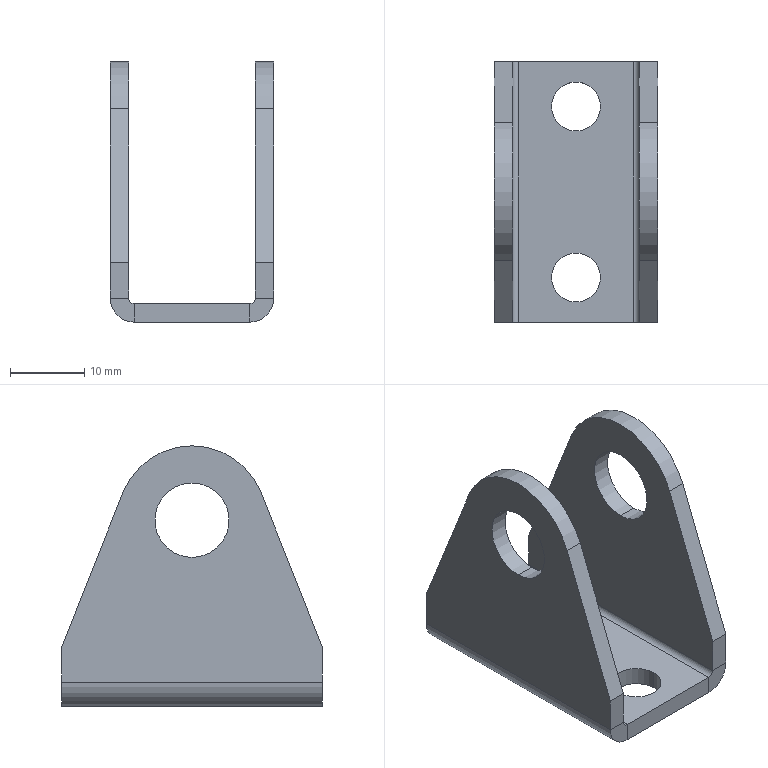Part | NX | features BREP 1 | 1 solid | 34 faces | box 22 x 35 x 35 mm | volume 5371 mm3 | plane 20 | cylinder 14 | commonest cylinder face diameters 6.6 x4 10 x4 1.473 x2 6.473 x2 20 x2
STEP:
#1=CARTESIAN_POINT('',(-3.3,-11.5,-2.5));
#2=VERTEX_POINT('',#1);
#3=CARTESIAN_POINT('',(3.3,-11.5,-2.5));
#4=VERTEX_POINT('',#3);
#5=CARTESIAN_POINT('',(0.,-11.5,-2.5));
#6=DIRECTION('',(0.,0.,1.));
#7=DIRECTION('',(1.,0.,0.));
#8=AXIS2_PLACEMENT_3D('',#5,#6,#7);
#9=CIRCLE('',#8,3.3);
#10=EDGE_CURVE('',#2,#4,#9,.T.);
#11=ORIENTED_EDGE('',*,*,#10,.F.);
#12=CARTESIAN_POINT('',(-3.3,-11.5,0.));
#13=VERTEX_POINT('',#12);
#14=CARTESIAN_POINT('',(-3.3,-11.5,0.));
#15=DIRECTION('',(0.,0.,1.));
#16=VECTOR('',#15,1000.);
#17=LINE('',#14,#16);
#18=EDGE_CURVE('',#13,#2,#17,.F.);
#19=ORIENTED_EDGE('',*,*,#18,.F.);
#20=CARTESIAN_POINT('',(3.3,-11.5,0.));
#21=VERTEX_POINT('',#20);
#22=CARTESIAN_POINT('',(0.,-11.5,0.));
#23=DIRECTION('',(0.,0.,1.));
#24=DIRECTION('',(1.,0.,0.));
#25=AXIS2_PLACEMENT_3D('',#22,#23,#24);
#26=CIRCLE('',#25,3.3);
#27=EDGE_CURVE('',#13,#21,#26,.T.);
#28=ORIENTED_EDGE('',*,*,#27,.T.);
#29=CARTESIAN_POINT('',(3.3,-11.5,0.));
#30=DIRECTION('',(0.,0.,1.));
#31=VECTOR('',#30,1000.);
#32=LINE('',#29,#31);
#33=EDGE_CURVE('',#21,#4,#32,.F.);
#34=ORIENTED_EDGE('',*,*,#33,.T.);
#35=EDGE_LOOP('',(#11,#19,#28,#34));
#36=FACE_BOUND('',#35,.T.);
#37=CARTESIAN_POINT('',(0.,-11.5,0.));
#38=DIRECTION('',(0.,0.,1.));
#39=DIRECTION('',(1.,0.,0.));
#40=AXIS2_PLACEMENT_3D('',#37,#38,#39);
#41=CYLINDRICAL_SURFACE('',#40,3.3);
#42=ADVANCED_FACE('',(#36),#41,.F.);
#43=CARTESIAN_POINT('',(-3.3,11.5,-2.5));
#44=VERTEX_POINT('',#43);
#45=CARTESIAN_POINT('',(3.3,11.5,-2.5));
#46=VERTEX_POINT('',#45);
#47=CARTESIAN_POINT('',(0.,11.5,-2.5));
#48=DIRECTION('',(0.,0.,1.));
#49=DIRECTION('',(1.,0.,0.));
#50=AXIS2_PLACEMENT_3D('',#47,#48,#49);
#51=CIRCLE('',#50,3.3);
#52=EDGE_CURVE('',#44,#46,#51,.T.);
#53=ORIENTED_EDGE('',*,*,#52,.F.);
#54=CARTESIAN_POINT('',(-3.3,11.5,0.));
#55=VERTEX_POINT('',#54);
#56=CARTESIAN_POINT('',(-3.3,11.5,0.));
#57=DIRECTION('',(0.,0.,1.));
#58=VECTOR('',#57,1000.);
#59=LINE('',#56,#58);
#60=EDGE_CURVE('',#55,#44,#59,.F.);
#61=ORIENTED_EDGE('',*,*,#60,.F.);
#62=CARTESIAN_POINT('',(3.3,11.5,0.));
#63=VERTEX_POINT('',#62);
#64=CARTESIAN_POINT('',(0.,11.5,0.));
#65=DIRECTION('',(0.,0.,1.));
#66=DIRECTION('',(1.,0.,0.));
#67=AXIS2_PLACEMENT_3D('',#64,#65,#66);
#68=CIRCLE('',#67,3.3);
#69=EDGE_CURVE('',#55,#63,#68,.T.);
#70=ORIENTED_EDGE('',*,*,#69,.T.);
#71=CARTESIAN_POINT('',(3.3,11.5,0.));
#72=DIRECTION('',(0.,0.,1.));
#73=VECTOR('',#72,1000.);
#74=LINE('',#71,#73);
#75=EDGE_CURVE('',#63,#46,#74,.F.);
#76=ORIENTED_EDGE('',*,*,#75,.T.);
#77=EDGE_LOOP('',(#53,#61,#70,#76));
#78=FACE_BOUND('',#77,.T.);
#79=CARTESIAN_POINT('',(0.,11.5,0.));
#80=DIRECTION('',(0.,0.,1.));
#81=DIRECTION('',(1.,0.,0.));
#82=AXIS2_PLACEMENT_3D('',#79,#80,#81);
#83=CYLINDRICAL_SURFACE('',#82,3.3);
#84=ADVANCED_FACE('',(#78),#83,.F.);
#85=CARTESIAN_POINT('',(-11.,0.,27.5));
#86=VERTEX_POINT('',#85);
#87=CARTESIAN_POINT('',(-11.,0.,17.5));
#88=VERTEX_POINT('',#87);
#89=CARTESIAN_POINT('',(-11.,0.,22.5));
#90=DIRECTION('',(1.,0.,0.));
#91=DIRECTION('',(0.,0.,-1.));
#92=AXIS2_PLACEMENT_3D('',#89,#90,#91);
#93=CIRCLE('',#92,5.);
#94=EDGE_CURVE('',#86,#88,#93,.T.);
#95=ORIENTED_EDGE('',*,*,#94,.F.);
#96=CARTESIAN_POINT('',(-8.5,0.,27.5));
#97=VERTEX_POINT('',#96);
#98=CARTESIAN_POINT('',(-29.,0.,27.5));
#99=DIRECTION('',(1.,0.,0.));
#100=VECTOR('',#99,1000.);
#101=LINE('',#98,#100);
#102=EDGE_CURVE('',#86,#97,#101,.T.);
#103=ORIENTED_EDGE('',*,*,#102,.T.);
#104=CARTESIAN_POINT('',(-8.5,0.,17.5));
#105=VERTEX_POINT('',#104);
#106=CARTESIAN_POINT('',(-8.5,0.,22.5));
#107=DIRECTION('',(1.,0.,0.));
#108=DIRECTION('',(0.,0.,-1.));
#109=AXIS2_PLACEMENT_3D('',#106,#107,#108);
#110=CIRCLE('',#109,5.);
#111=EDGE_CURVE('',#97,#105,#110,.T.);
#112=ORIENTED_EDGE('',*,*,#111,.T.);
#113=CARTESIAN_POINT('',(-29.,0.,17.5));
#114=DIRECTION('',(1.,0.,0.));
#115=VECTOR('',#114,1000.);
#116=LINE('',#113,#115);
#117=EDGE_CURVE('',#88,#105,#116,.T.);
#118=ORIENTED_EDGE('',*,*,#117,.F.);
#119=EDGE_LOOP('',(#95,#103,#112,#118));
#120=FACE_BOUND('',#119,.T.);
#121=CARTESIAN_POINT('',(-29.,0.,22.5));
#122=DIRECTION('',(1.,0.,0.));
#123=DIRECTION('',(0.,0.,-1.));
#124=AXIS2_PLACEMENT_3D('',#121,#122,#123);
#125=CYLINDRICAL_SURFACE('',#124,5.);
#126=ADVANCED_FACE('',(#120),#125,.F.);
#127=CARTESIAN_POINT('',(8.5,0.,17.5));
#128=VERTEX_POINT('',#127);
#129=CARTESIAN_POINT('',(8.5,0.,27.5));
#130=VERTEX_POINT('',#129);
#131=CARTESIAN_POINT('',(8.5,0.,22.5));
#132=DIRECTION('',(-1.,0.,0.));
#133=DIRECTION('',(0.,0.,1.));
#134=AXIS2_PLACEMENT_3D('',#131,#132,#133);
#135=CIRCLE('',#134,5.);
#136=EDGE_CURVE('',#128,#130,#135,.T.);
#137=ORIENTED_EDGE('',*,*,#136,.T.);
#138=CARTESIAN_POINT('',(11.,0.,27.5));
#139=VERTEX_POINT('',#138);
#140=CARTESIAN_POINT('',(-29.,0.,27.5));
#141=DIRECTION('',(1.,0.,0.));
#142=VECTOR('',#141,1000.);
#143=LINE('',#140,#142);
#144=EDGE_CURVE('',#130,#139,#143,.T.);
#145=ORIENTED_EDGE('',*,*,#144,.T.);
#146=CARTESIAN_POINT('',(11.,0.,17.5));
#147=VERTEX_POINT('',#146);
#148=CARTESIAN_POINT('',(11.,0.,22.5));
#149=DIRECTION('',(1.,0.,0.));
#150=DIRECTION('',(0.,0.,-1.));
#151=AXIS2_PLACEMENT_3D('',#148,#149,#150);
#152=CIRCLE('',#151,5.);
#153=EDGE_CURVE('',#139,#147,#152,.T.);
#154=ORIENTED_EDGE('',*,*,#153,.T.);
#155=CARTESIAN_POINT('',(-29.,0.,17.5));
#156=DIRECTION('',(1.,0.,0.));
#157=VECTOR('',#156,1000.);
#158=LINE('',#155,#157);
#159=EDGE_CURVE('',#128,#147,#158,.T.);
#160=ORIENTED_EDGE('',*,*,#159,.F.);
#161=EDGE_LOOP('',(#137,#145,#154,#160));
#162=FACE_BOUND('',#161,.T.);
#163=CARTESIAN_POINT('',(-29.,0.,22.5));
#164=DIRECTION('',(1.,0.,0.));
#165=DIRECTION('',(0.,0.,-1.));
#166=AXIS2_PLACEMENT_3D('',#163,#164,#165);
#167=CYLINDRICAL_SURFACE('',#166,5.);
#168=ADVANCED_FACE('',(#162),#167,.F.);
#169=CARTESIAN_POINT('',(7.763,17.5,-2.5));
#170=VERTEX_POINT('',#169);
#171=CARTESIAN_POINT('',(-7.763,17.5,-2.5));
#172=VERTEX_POINT('',#171);
#173=CARTESIAN_POINT('',(-11.,17.5,-2.5));
#174=DIRECTION('',(-1.,0.,0.));
#175=VECTOR('',#174,1000.);
#176=LINE('',#173,#175);
#177=EDGE_CURVE('',#170,#172,#176,.T.);
#178=ORIENTED_EDGE('',*,*,#177,.F.);
#179=CARTESIAN_POINT('',(7.763,-17.5,-2.5));
#180=VERTEX_POINT('',#179);
#181=CARTESIAN_POINT('',(7.763,17.5,-2.5));
#182=DIRECTION('',(0.,-1.,0.));
#183=VECTOR('',#182,1000.);
#184=LINE('',#181,#183);
#185=EDGE_CURVE('',#170,#180,#184,.T.);
#186=ORIENTED_EDGE('',*,*,#185,.T.);
#187=CARTESIAN_POINT('',(-7.763,-17.5,-2.5));
#188=VERTEX_POINT('',#187);
#189=CARTESIAN_POINT('',(-11.,-17.5,-2.5));
#190=DIRECTION('',(1.,0.,0.));
#191=VECTOR('',#190,1000.);
#192=LINE('',#189,#191);
#193=EDGE_CURVE('',#188,#180,#192,.T.);
#194=ORIENTED_EDGE('',*,*,#193,.F.);
#195=CARTESIAN_POINT('',(-7.763,-17.5,-2.5));
#196=DIRECTION('',(0.,1.,0.));
#197=VECTOR('',#196,1000.);
#198=LINE('',#195,#197);
#199=EDGE_CURVE('',#188,#172,#198,.T.);
#200=ORIENTED_EDGE('',*,*,#199,.T.);
#201=EDGE_LOOP('',(#178,#186,#194,#200));
#202=FACE_BOUND('',#201,.T.);
#203=CARTESIAN_POINT('',(0.,11.5,-2.5));
#204=DIRECTION('',(0.,0.,1.));
#205=DIRECTION('',(1.,0.,0.));
#206=AXIS2_PLACEMENT_3D('',#203,#204,#205);
#207=CIRCLE('',#206,3.3);
#208=EDGE_CURVE('',#46,#44,#207,.T.);
#209=ORIENTED_EDGE('',*,*,#208,.T.);
#210=ORIENTED_EDGE('',*,*,#52,.T.);
#211=EDGE_LOOP('',(#209,#210));
#212=FACE_BOUND('',#211,.T.);
#213=CARTESIAN_POINT('',(0.,-11.5,-2.5));
#214=DIRECTION('',(0.,0.,1.));
#215=DIRECTION('',(1.,0.,0.));
#216=AXIS2_PLACEMENT_3D('',#213,#214,#215);
#217=CIRCLE('',#216,3.3);
#218=EDGE_CURVE('',#4,#2,#217,.T.);
#219=ORIENTED_EDGE('',*,*,#218,.T.);
#220=ORIENTED_EDGE('',*,*,#10,.T.);
#221=EDGE_LOOP('',(#219,#220));
#222=FACE_BOUND('',#221,.T.);
#223=CARTESIAN_POINT('',(0.,0.,-2.5));
#224=DIRECTION('',(0.,0.,-1.));
#225=DIRECTION('',(0.,-1.,0.));
#226=AXIS2_PLACEMENT_3D('',#223,#224,#225);
#227=PLANE('',#226);
#228=ADVANCED_FACE('',(#202,#212,#222),#227,.T.);
#229=CARTESIAN_POINT('',(7.763,17.5,0.));
#230=VERTEX_POINT('',#229);
#231=CARTESIAN_POINT('',(7.763,-17.5,0.));
#232=VERTEX_POINT('',#231);
#233=CARTESIAN_POINT('',(7.763,17.5,0.));
#234=DIRECTION('',(0.,-1.,0.));
#235=VECTOR('',#234,1000.);
#236=LINE('',#233,#235);
#237=EDGE_CURVE('',#230,#232,#236,.T.);
#238=ORIENTED_EDGE('',*,*,#237,.F.);
#239=CARTESIAN_POINT('',(-7.763,17.5,0.));
#240=VERTEX_POINT('',#239);
#241=CARTESIAN_POINT('',(-11.,17.5,0.));
#242=DIRECTION('',(-1.,0.,0.));
#243=VECTOR('',#242,1000.);
#244=LINE('',#241,#243);
#245=EDGE_CURVE('',#230,#240,#244,.T.);
#246=ORIENTED_EDGE('',*,*,#245,.T.);
#247=CARTESIAN_POINT('',(-7.763,-17.5,0.));
#248=VERTEX_POINT('',#247);
#249=CARTESIAN_POINT('',(-7.763,-17.5,0.));
#250=DIRECTION('',(0.,1.,0.));
#251=VECTOR('',#250,1000.);
#252=LINE('',#249,#251);
#253=EDGE_CURVE('',#248,#240,#252,.T.);
#254=ORIENTED_EDGE('',*,*,#253,.F.);
#255=CARTESIAN_POINT('',(-11.,-17.5,0.));
#256=DIRECTION('',(1.,0.,0.));
#257=VECTOR('',#256,1000.);
#258=LINE('',#255,#257);
#259=EDGE_CURVE('',#248,#232,#258,.T.);
#260=ORIENTED_EDGE('',*,*,#259,.T.);
#261=EDGE_LOOP('',(#238,#246,#254,#260));
#262=FACE_BOUND('',#261,.T.);
#263=CARTESIAN_POINT('',(0.,-11.5,0.));
#264=DIRECTION('',(0.,0.,1.));
#265=DIRECTION('',(1.,0.,0.));
#266=AXIS2_PLACEMENT_3D('',#263,#264,#265);
#267=CIRCLE('',#266,3.3);
#268=EDGE_CURVE('',#21,#13,#267,.T.);
#269=ORIENTED_EDGE('',*,*,#268,.F.);
#270=ORIENTED_EDGE('',*,*,#27,.F.);
#271=EDGE_LOOP('',(#269,#270));
#272=FACE_BOUND('',#271,.T.);
#273=CARTESIAN_POINT('',(0.,11.5,0.));
#274=DIRECTION('',(0.,0.,1.));
#275=DIRECTION('',(1.,0.,0.));
#276=AXIS2_PLACEMENT_3D('',#273,#274,#275);
#277=CIRCLE('',#276,3.3);
#278=EDGE_CURVE('',#63,#55,#277,.T.);
#279=ORIENTED_EDGE('',*,*,#278,.F.);
#280=ORIENTED_EDGE('',*,*,#69,.F.);
#281=EDGE_LOOP('',(#279,#280));
#282=FACE_BOUND('',#281,.T.);
#283=CARTESIAN_POINT('',(0.,0.,0.));
#284=DIRECTION('',(0.,0.,-1.));
#285=DIRECTION('',(0.,-1.,0.));
#286=AXIS2_PLACEMENT_3D('',#283,#284,#285);
#287=PLANE('',#286);
#288=ADVANCED_FACE('',(#262,#272,#282),#287,.F.);
#289=ORIENTED_EDGE('',*,*,#245,.F.);
#290=CARTESIAN_POINT('',(7.763,17.5,0.));
#291=DIRECTION('',(0.,0.,-1.));
#292=VECTOR('',#291,1000.);
#293=LINE('',#290,#292);
#294=EDGE_CURVE('',#230,#170,#293,.T.);
#295=ORIENTED_EDGE('',*,*,#294,.T.);
#296=ORIENTED_EDGE('',*,*,#177,.T.);
#297=CARTESIAN_POINT('',(-7.763,17.5,0.));
#298=DIRECTION('',(0.,0.,-1.));
#299=VECTOR('',#298,1000.);
#300=LINE('',#297,#299);
#301=EDGE_CURVE('',#240,#172,#300,.T.);
#302=ORIENTED_EDGE('',*,*,#301,.F.);
#303=EDGE_LOOP('',(#289,#295,#296,#302));
#304=FACE_BOUND('',#303,.T.);
#305=CARTESIAN_POINT('',(-11.,17.5,-2.5));
#306=DIRECTION('',(0.,1.,0.));
#307=DIRECTION('',(1.,0.,0.));
#308=AXIS2_PLACEMENT_3D('',#305,#306,#307);
#309=PLANE('',#308);
#310=ADVANCED_FACE('',(#304),#309,.T.);
#311=CARTESIAN_POINT('',(7.763,-17.5,0.));
#312=DIRECTION('',(0.,0.,-1.));
#313=VECTOR('',#312,1000.);
#314=LINE('',#311,#313);
#315=EDGE_CURVE('',#232,#180,#314,.T.);
#316=ORIENTED_EDGE('',*,*,#315,.F.);
#317=ORIENTED_EDGE('',*,*,#259,.F.);
#318=CARTESIAN_POINT('',(-7.763,-17.5,0.));
#319=DIRECTION('',(0.,0.,-1.));
#320=VECTOR('',#319,1000.);
#321=LINE('',#318,#320);
#322=EDGE_CURVE('',#248,#188,#321,.T.);
#323=ORIENTED_EDGE('',*,*,#322,.T.);
#324=ORIENTED_EDGE('',*,*,#193,.T.);
#325=EDGE_LOOP('',(#316,#317,#323,#324));
#326=FACE_BOUND('',#325,.T.);
#327=CARTESIAN_POINT('',(-11.,-17.5,-2.5));
#328=DIRECTION('',(0.,-1.,0.));
#329=DIRECTION('',(0.,0.,-1.));
#330=AXIS2_PLACEMENT_3D('',#327,#328,#329);
#331=PLANE('',#330);
#332=ADVANCED_FACE('',(#326),#331,.T.);
#333=CARTESIAN_POINT('',(-8.5,17.5,0.7366));
#334=VERTEX_POINT('',#333);
#335=CARTESIAN_POINT('',(-11.,17.5,0.7366));
#336=VERTEX_POINT('',#335);
#337=CARTESIAN_POINT('',(-11.,17.5,0.7366));
#338=DIRECTION('',(-1.,0.,0.));
#339=VECTOR('',#338,1000.);
#340=LINE('',#337,#339);
#341=EDGE_CURVE('',#334,#336,#340,.T.);
#342=ORIENTED_EDGE('',*,*,#341,.F.);
#343=CARTESIAN_POINT('',(-7.763,17.5,0.7366));
#344=DIRECTION('',(0.,1.,0.));
#345=DIRECTION('',(0.,0.,-1.));
#346=AXIS2_PLACEMENT_3D('',#343,#344,#345);
#347=CIRCLE('',#346,0.7366);
#348=EDGE_CURVE('',#240,#334,#347,.T.);
#349=ORIENTED_EDGE('',*,*,#348,.F.);
#350=ORIENTED_EDGE('',*,*,#301,.T.);
#351=CARTESIAN_POINT('',(-7.763,17.5,0.7366));
#352=DIRECTION('',(0.,1.,0.));
#353=DIRECTION('',(0.,0.,-1.));
#354=AXIS2_PLACEMENT_3D('',#351,#352,#353);
#355=CIRCLE('',#354,3.237);
#356=EDGE_CURVE('',#172,#336,#355,.T.);
#357=ORIENTED_EDGE('',*,*,#356,.T.);
#358=EDGE_LOOP('',(#342,#349,#350,#357));
#359=FACE_BOUND('',#358,.T.);
#360=CARTESIAN_POINT('',(-7.763,17.5,0.7366));
#361=DIRECTION('',(0.,1.,0.));
#362=DIRECTION('',(1.,0.,0.));
#363=AXIS2_PLACEMENT_3D('',#360,#361,#362);
#364=PLANE('',#363);
#365=ADVANCED_FACE('',(#359),#364,.T.);
#366=CARTESIAN_POINT('',(-8.5,-17.5,0.7366));
#367=VERTEX_POINT('',#366);
#368=CARTESIAN_POINT('',(-7.763,-17.5,0.7366));
#369=DIRECTION('',(0.,-1.,0.));
#370=DIRECTION('',(0.,0.,-1.));
#371=AXIS2_PLACEMENT_3D('',#368,#369,#370);
#372=CIRCLE('',#371,0.7366);
#373=EDGE_CURVE('',#367,#248,#372,.T.);
#374=ORIENTED_EDGE('',*,*,#373,.F.);
#375=CARTESIAN_POINT('',(-11.,-17.5,0.7366));
#376=VERTEX_POINT('',#375);
#377=CARTESIAN_POINT('',(-8.5,-17.5,0.7366));
#378=DIRECTION('',(-1.,0.,0.));
#379=VECTOR('',#378,1000.);
#380=LINE('',#377,#379);
#381=EDGE_CURVE('',#367,#376,#380,.T.);
#382=ORIENTED_EDGE('',*,*,#381,.T.);
#383=CARTESIAN_POINT('',(-7.763,-17.5,0.7366));
#384=DIRECTION('',(0.,-1.,0.));
#385=DIRECTION('',(0.,0.,-1.));
#386=AXIS2_PLACEMENT_3D('',#383,#384,#385);
#387=CIRCLE('',#386,3.237);
#388=EDGE_CURVE('',#376,#188,#387,.T.);
#389=ORIENTED_EDGE('',*,*,#388,.T.);
#390=ORIENTED_EDGE('',*,*,#322,.F.);
#391=EDGE_LOOP('',(#374,#382,#389,#390));
#392=FACE_BOUND('',#391,.T.);
#393=CARTESIAN_POINT('',(-7.763,-17.5,0.7366));
#394=DIRECTION('',(0.,1.,0.));
#395=DIRECTION('',(1.,0.,0.));
#396=AXIS2_PLACEMENT_3D('',#393,#394,#395);
#397=PLANE('',#396);
#398=ADVANCED_FACE('',(#392),#397,.F.);
#399=ORIENTED_EDGE('',*,*,#199,.F.);
#400=ORIENTED_EDGE('',*,*,#388,.F.);
#401=CARTESIAN_POINT('',(-11.,17.5,0.7366));
#402=DIRECTION('',(0.,1.,0.));
#403=VECTOR('',#402,1000.);
#404=LINE('',#401,#403);
#405=EDGE_CURVE('',#376,#336,#404,.T.);
#406=ORIENTED_EDGE('',*,*,#405,.T.);
#407=ORIENTED_EDGE('',*,*,#356,.F.);
#408=EDGE_LOOP('',(#399,#400,#406,#407));
#409=FACE_BOUND('',#408,.T.);
#410=CARTESIAN_POINT('',(-7.763,-17.5,0.7366));
#411=DIRECTION('',(0.,-1.,0.));
#412=DIRECTION('',(-1.,0.,0.));
#413=AXIS2_PLACEMENT_3D('',#410,#411,#412);
#414=CYLINDRICAL_SURFACE('',#413,3.237);
#415=ADVANCED_FACE('',(#409),#414,.T.);
#416=ORIENTED_EDGE('',*,*,#253,.T.);
#417=ORIENTED_EDGE('',*,*,#348,.T.);
#418=CARTESIAN_POINT('',(-8.5,17.5,0.7366));
#419=DIRECTION('',(0.,-1.,0.));
#420=VECTOR('',#419,1000.);
#421=LINE('',#418,#420);
#422=EDGE_CURVE('',#334,#367,#421,.T.);
#423=ORIENTED_EDGE('',*,*,#422,.T.);
#424=ORIENTED_EDGE('',*,*,#373,.T.);
#425=EDGE_LOOP('',(#416,#417,#423,#424));
#426=FACE_BOUND('',#425,.T.);
#427=CARTESIAN_POINT('',(-7.763,-17.5,0.7366));
#428=DIRECTION('',(0.,-1.,0.));
#429=DIRECTION('',(-1.,0.,0.));
#430=AXIS2_PLACEMENT_3D('',#427,#428,#429);
#431=CYLINDRICAL_SURFACE('',#430,0.7366);
#432=ADVANCED_FACE('',(#426),#431,.F.);
#433=CARTESIAN_POINT('',(-11.,17.5,5.5));
#434=VERTEX_POINT('',#433);
#435=CARTESIAN_POINT('',(-11.,17.5,0.));
#436=DIRECTION('',(0.,0.,-1.));
#437=VECTOR('',#436,1000.);
#438=LINE('',#435,#437);
#439=EDGE_CURVE('',#434,#336,#438,.T.);
#440=ORIENTED_EDGE('',*,*,#439,.F.);
#441=CARTESIAN_POINT('',(-8.5,17.5,5.5));
#442=VERTEX_POINT('',#441);
#443=CARTESIAN_POINT('',(-29.,17.5,5.5));
#444=DIRECTION('',(1.,0.,0.));
#445=VECTOR('',#444,1000.);
#446=LINE('',#443,#445);
#447=EDGE_CURVE('',#434,#442,#446,.T.);
#448=ORIENTED_EDGE('',*,*,#447,.T.);
#449=CARTESIAN_POINT('',(-8.5,17.5,0.));
#450=DIRECTION('',(0.,0.,-1.));
#451=VECTOR('',#450,1000.);
#452=LINE('',#449,#451);
#453=EDGE_CURVE('',#442,#334,#452,.T.);
#454=ORIENTED_EDGE('',*,*,#453,.T.);
#455=ORIENTED_EDGE('',*,*,#341,.T.);
#456=EDGE_LOOP('',(#440,#448,#454,#455));
#457=FACE_BOUND('',#456,.T.);
#458=CARTESIAN_POINT('',(-11.,17.5,0.));
#459=DIRECTION('',(0.,-1.,0.));
#460=DIRECTION('',(0.,0.,-1.));
#461=AXIS2_PLACEMENT_3D('',#458,#459,#460);
#462=PLANE('',#461);
#463=ADVANCED_FACE('',(#457),#462,.F.);
#464=CARTESIAN_POINT('',(-8.5,-17.5,5.5));
#465=VERTEX_POINT('',#464);
#466=CARTESIAN_POINT('',(-8.5,-17.5,37.5));
#467=DIRECTION('',(0.,0.,1.));
#468=VECTOR('',#467,1000.);
#469=LINE('',#466,#468);
#470=EDGE_CURVE('',#367,#465,#469,.T.);
#471=ORIENTED_EDGE('',*,*,#470,.T.);
#472=CARTESIAN_POINT('',(-11.,-17.5,5.5));
#473=VERTEX_POINT('',#472);
#474=CARTESIAN_POINT('',(-29.,-17.5,5.5));
#475=DIRECTION('',(1.,0.,0.));
#476=VECTOR('',#475,1000.);
#477=LINE('',#474,#476);
#478=EDGE_CURVE('',#473,#465,#477,.T.);
#479=ORIENTED_EDGE('',*,*,#478,.F.);
#480=CARTESIAN_POINT('',(-11.,-17.5,0.));
#481=DIRECTION('',(0.,0.,1.));
#482=VECTOR('',#481,1000.);
#483=LINE('',#480,#482);
#484=EDGE_CURVE('',#376,#473,#483,.T.);
#485=ORIENTED_EDGE('',*,*,#484,.F.);
#486=ORIENTED_EDGE('',*,*,#381,.F.);
#487=EDGE_LOOP('',(#471,#479,#485,#486));
#488=FACE_BOUND('',#487,.T.);
#489=CARTESIAN_POINT('',(-11.,-17.5,37.5));
#490=DIRECTION('',(0.,1.,0.));
#491=DIRECTION('',(1.,0.,0.));
#492=AXIS2_PLACEMENT_3D('',#489,#490,#491);
#493=PLANE('',#492);
#494=ADVANCED_FACE('',(#488),#493,.F.);
#495=ORIENTED_EDGE('',*,*,#484,.T.);
#496=CARTESIAN_POINT('',(-11.,-9.296,26.187));
#497=VERTEX_POINT('',#496);
#498=CARTESIAN_POINT('',(-11.,-17.006,6.745));
#499=DIRECTION('',(0.,0.3687,0.9296));
#500=VECTOR('',#499,1000.);
#501=LINE('',#498,#500);
#502=EDGE_CURVE('',#473,#497,#501,.T.);
#503=ORIENTED_EDGE('',*,*,#502,.T.);
#504=CARTESIAN_POINT('',(-11.,9.296,26.187));
#505=VERTEX_POINT('',#504);
#506=CARTESIAN_POINT('',(-11.,0.,22.5));
#507=DIRECTION('',(-1.,0.,0.));
#508=DIRECTION('',(0.,0.,-1.));
#509=AXIS2_PLACEMENT_3D('',#506,#507,#508);
#510=CIRCLE('',#509,10.);
#511=EDGE_CURVE('',#497,#505,#510,.T.);
#512=ORIENTED_EDGE('',*,*,#511,.T.);
#513=CARTESIAN_POINT('',(-11.,17.006,6.745));
#514=DIRECTION('',(0.,0.3687,-0.9296));
#515=VECTOR('',#514,1000.);
#516=LINE('',#513,#515);
#517=EDGE_CURVE('',#505,#434,#516,.T.);
#518=ORIENTED_EDGE('',*,*,#517,.T.);
#519=ORIENTED_EDGE('',*,*,#439,.T.);
#520=ORIENTED_EDGE('',*,*,#405,.F.);
#521=EDGE_LOOP('',(#495,#503,#512,#518,#519,#520));
#522=FACE_BOUND('',#521,.T.);
#523=CARTESIAN_POINT('',(-11.,0.,22.5));
#524=DIRECTION('',(1.,0.,0.));
#525=DIRECTION('',(0.,0.,-1.));
#526=AXIS2_PLACEMENT_3D('',#523,#524,#525);
#527=CIRCLE('',#526,5.);
#528=EDGE_CURVE('',#88,#86,#527,.T.);
#529=ORIENTED_EDGE('',*,*,#528,.T.);
#530=ORIENTED_EDGE('',*,*,#94,.T.);
#531=EDGE_LOOP('',(#529,#530));
#532=FACE_BOUND('',#531,.T.);
#533=CARTESIAN_POINT('',(-11.,0.,0.));
#534=DIRECTION('',(1.,0.,0.));
#535=DIRECTION('',(0.,0.,1.));
#536=AXIS2_PLACEMENT_3D('',#533,#534,#535);
#537=PLANE('',#536);
#538=ADVANCED_FACE('',(#522,#532),#537,.F.);
#539=CARTESIAN_POINT('',(-8.5,-9.296,26.187));
#540=VERTEX_POINT('',#539);
#541=CARTESIAN_POINT('',(-8.5,-17.006,6.745));
#542=DIRECTION('',(0.,0.3687,0.9296));
#543=VECTOR('',#542,1000.);
#544=LINE('',#541,#543);
#545=EDGE_CURVE('',#465,#540,#544,.T.);
#546=ORIENTED_EDGE('',*,*,#545,.F.);
#547=ORIENTED_EDGE('',*,*,#470,.F.);
#548=ORIENTED_EDGE('',*,*,#422,.F.);
#549=ORIENTED_EDGE('',*,*,#453,.F.);
#550=CARTESIAN_POINT('',(-8.5,9.296,26.187));
#551=VERTEX_POINT('',#550);
#552=CARTESIAN_POINT('',(-8.5,17.006,6.745));
#553=DIRECTION('',(0.,0.3687,-0.9296));
#554=VECTOR('',#553,1000.);
#555=LINE('',#552,#554);
#556=EDGE_CURVE('',#551,#442,#555,.T.);
#557=ORIENTED_EDGE('',*,*,#556,.F.);
#558=CARTESIAN_POINT('',(-8.5,0.,22.5));
#559=DIRECTION('',(-1.,0.,0.));
#560=DIRECTION('',(0.,0.,-1.));
#561=AXIS2_PLACEMENT_3D('',#558,#559,#560);
#562=CIRCLE('',#561,10.);
#563=EDGE_CURVE('',#540,#551,#562,.T.);
#564=ORIENTED_EDGE('',*,*,#563,.F.);
#565=EDGE_LOOP('',(#546,#547,#548,#549,#557,#564));
#566=FACE_BOUND('',#565,.T.);
#567=CARTESIAN_POINT('',(-8.5,0.,22.5));
#568=DIRECTION('',(1.,0.,0.));
#569=DIRECTION('',(0.,0.,-1.));
#570=AXIS2_PLACEMENT_3D('',#567,#568,#569);
#571=CIRCLE('',#570,5.);
#572=EDGE_CURVE('',#105,#97,#571,.T.);
#573=ORIENTED_EDGE('',*,*,#572,.F.);
#574=ORIENTED_EDGE('',*,*,#111,.F.);
#575=EDGE_LOOP('',(#573,#574));
#576=FACE_BOUND('',#575,.T.);
#577=CARTESIAN_POINT('',(-8.5,0.,0.));
#578=DIRECTION('',(1.,0.,0.));
#579=DIRECTION('',(0.,0.,1.));
#580=AXIS2_PLACEMENT_3D('',#577,#578,#579);
#581=PLANE('',#580);
#582=ADVANCED_FACE('',(#566,#576),#581,.T.);
#583=CARTESIAN_POINT('',(8.5,-17.5,0.7366));
#584=VERTEX_POINT('',#583);
#585=CARTESIAN_POINT('',(11.,-17.5,0.7366));
#586=VERTEX_POINT('',#585);
#587=CARTESIAN_POINT('',(11.,-17.5,0.7366));
#588=DIRECTION('',(1.,0.,0.));
#589=VECTOR('',#588,1000.);
#590=LINE('',#587,#589);
#591=EDGE_CURVE('',#584,#586,#590,.T.);
#592=ORIENTED_EDGE('',*,*,#591,.F.);
#593=CARTESIAN_POINT('',(7.763,-17.5,0.7366));
#594=DIRECTION('',(0.,-1.,0.));
#595=DIRECTION('',(0.,0.,1.));
#596=AXIS2_PLACEMENT_3D('',#593,#594,#595);
#597=CIRCLE('',#596,0.7366);
#598=EDGE_CURVE('',#232,#584,#597,.T.);
#599=ORIENTED_EDGE('',*,*,#598,.F.);
#600=ORIENTED_EDGE('',*,*,#315,.T.);
#601=CARTESIAN_POINT('',(7.763,-17.5,0.7366));
#602=DIRECTION('',(0.,-1.,0.));
#603=DIRECTION('',(0.,0.,1.));
#604=AXIS2_PLACEMENT_3D('',#601,#602,#603);
#605=CIRCLE('',#604,3.237);
#606=EDGE_CURVE('',#180,#586,#605,.T.);
#607=ORIENTED_EDGE('',*,*,#606,.T.);
#608=EDGE_LOOP('',(#592,#599,#600,#607));
#609=FACE_BOUND('',#608,.T.);
#610=CARTESIAN_POINT('',(7.763,-17.5,0.7366));
#611=DIRECTION('',(0.,-1.,0.));
#612=DIRECTION('',(0.,0.,-1.));
#613=AXIS2_PLACEMENT_3D('',#610,#611,#612);
#614=PLANE('',#613);
#615=ADVANCED_FACE('',(#609),#614,.T.);
#616=CARTESIAN_POINT('',(8.5,17.5,0.7366));
#617=VERTEX_POINT('',#616);
#618=CARTESIAN_POINT('',(7.763,17.5,0.7366));
#619=DIRECTION('',(0.,1.,0.));
#620=DIRECTION('',(0.,0.,1.));
#621=AXIS2_PLACEMENT_3D('',#618,#619,#620);
#622=CIRCLE('',#621,0.7366);
#623=EDGE_CURVE('',#617,#230,#622,.T.);
#624=ORIENTED_EDGE('',*,*,#623,.F.);
#625=CARTESIAN_POINT('',(11.,17.5,0.7366));
#626=VERTEX_POINT('',#625);
#627=CARTESIAN_POINT('',(8.5,17.5,0.7366));
#628=DIRECTION('',(1.,0.,0.));
#629=VECTOR('',#628,1000.);
#630=LINE('',#627,#629);
#631=EDGE_CURVE('',#617,#626,#630,.T.);
#632=ORIENTED_EDGE('',*,*,#631,.T.);
#633=CARTESIAN_POINT('',(7.763,17.5,0.7366));
#634=DIRECTION('',(0.,1.,0.));
#635=DIRECTION('',(0.,0.,1.));
#636=AXIS2_PLACEMENT_3D('',#633,#634,#635);
#637=CIRCLE('',#636,3.237);
#638=EDGE_CURVE('',#626,#170,#637,.T.);
#639=ORIENTED_EDGE('',*,*,#638,.T.);
#640=ORIENTED_EDGE('',*,*,#294,.F.);
#641=EDGE_LOOP('',(#624,#632,#639,#640));
#642=FACE_BOUND('',#641,.T.);
#643=CARTESIAN_POINT('',(7.763,17.5,0.7366));
#644=DIRECTION('',(0.,-1.,0.));
#645=DIRECTION('',(0.,0.,-1.));
#646=AXIS2_PLACEMENT_3D('',#643,#644,#645);
#647=PLANE('',#646);
#648=ADVANCED_FACE('',(#642),#647,.F.);
#649=ORIENTED_EDGE('',*,*,#185,.F.);
#650=ORIENTED_EDGE('',*,*,#638,.F.);
#651=CARTESIAN_POINT('',(11.,-17.5,0.7366));
#652=DIRECTION('',(0.,-1.,0.));
#653=VECTOR('',#652,1000.);
#654=LINE('',#651,#653);
#655=EDGE_CURVE('',#626,#586,#654,.T.);
#656=ORIENTED_EDGE('',*,*,#655,.T.);
#657=ORIENTED_EDGE('',*,*,#606,.F.);
#658=EDGE_LOOP('',(#649,#650,#656,#657));
#659=FACE_BOUND('',#658,.T.);
#660=CARTESIAN_POINT('',(7.763,17.5,0.7366));
#661=DIRECTION('',(0.,1.,0.));
#662=DIRECTION('',(1.,0.,0.));
#663=AXIS2_PLACEMENT_3D('',#660,#661,#662);
#664=CYLINDRICAL_SURFACE('',#663,3.237);
#665=ADVANCED_FACE('',(#659),#664,.T.);
#666=ORIENTED_EDGE('',*,*,#237,.T.);
#667=ORIENTED_EDGE('',*,*,#598,.T.);
#668=CARTESIAN_POINT('',(8.5,-17.5,0.7366));
#669=DIRECTION('',(0.,1.,0.));
#670=VECTOR('',#669,1000.);
#671=LINE('',#668,#670);
#672=EDGE_CURVE('',#584,#617,#671,.T.);
#673=ORIENTED_EDGE('',*,*,#672,.T.);
#674=ORIENTED_EDGE('',*,*,#623,.T.);
#675=EDGE_LOOP('',(#666,#667,#673,#674));
#676=FACE_BOUND('',#675,.T.);
#677=CARTESIAN_POINT('',(7.763,17.5,0.7366));
#678=DIRECTION('',(0.,1.,0.));
#679=DIRECTION('',(1.,0.,0.));
#680=AXIS2_PLACEMENT_3D('',#677,#678,#679);
#681=CYLINDRICAL_SURFACE('',#680,0.7366);
#682=ADVANCED_FACE('',(#676),#681,.F.);
#683=CARTESIAN_POINT('',(11.,-17.5,5.5));
#684=VERTEX_POINT('',#683);
#685=CARTESIAN_POINT('',(11.,-17.5,0.));
#686=DIRECTION('',(0.,0.,-1.));
#687=VECTOR('',#686,1000.);
#688=LINE('',#685,#687);
#689=EDGE_CURVE('',#684,#586,#688,.T.);
#690=ORIENTED_EDGE('',*,*,#689,.F.);
#691=CARTESIAN_POINT('',(8.5,-17.5,5.5));
#692=VERTEX_POINT('',#691);
#693=CARTESIAN_POINT('',(-29.,-17.5,5.5));
#694=DIRECTION('',(1.,0.,0.));
#695=VECTOR('',#694,1000.);
#696=LINE('',#693,#695);
#697=EDGE_CURVE('',#692,#684,#696,.T.);
#698=ORIENTED_EDGE('',*,*,#697,.F.);
#699=CARTESIAN_POINT('',(8.5,-17.5,0.));
#700=DIRECTION('',(0.,0.,-1.));
#701=VECTOR('',#700,1000.);
#702=LINE('',#699,#701);
#703=EDGE_CURVE('',#692,#584,#702,.T.);
#704=ORIENTED_EDGE('',*,*,#703,.T.);
#705=ORIENTED_EDGE('',*,*,#591,.T.);
#706=EDGE_LOOP('',(#690,#698,#704,#705));
#707=FACE_BOUND('',#706,.T.);
#708=CARTESIAN_POINT('',(11.,-17.5,0.));
#709=DIRECTION('',(0.,1.,0.));
#710=DIRECTION('',(0.,0.,-1.));
#711=AXIS2_PLACEMENT_3D('',#708,#709,#710);
#712=PLANE('',#711);
#713=ADVANCED_FACE('',(#707),#712,.F.);
#714=CARTESIAN_POINT('',(8.5,17.5,5.5));
#715=VERTEX_POINT('',#714);
#716=CARTESIAN_POINT('',(8.5,17.5,37.5));
#717=DIRECTION('',(0.,0.,1.));
#718=VECTOR('',#717,1000.);
#719=LINE('',#716,#718);
#720=EDGE_CURVE('',#617,#715,#719,.T.);
#721=ORIENTED_EDGE('',*,*,#720,.T.);
#722=CARTESIAN_POINT('',(11.,17.5,5.5));
#723=VERTEX_POINT('',#722);
#724=CARTESIAN_POINT('',(-29.,17.5,5.5));
#725=DIRECTION('',(1.,0.,0.));
#726=VECTOR('',#725,1000.);
#727=LINE('',#724,#726);
#728=EDGE_CURVE('',#715,#723,#727,.T.);
#729=ORIENTED_EDGE('',*,*,#728,.T.);
#730=CARTESIAN_POINT('',(11.,17.5,0.));
#731=DIRECTION('',(0.,0.,1.));
#732=VECTOR('',#731,1000.);
#733=LINE('',#730,#732);
#734=EDGE_CURVE('',#626,#723,#733,.T.);
#735=ORIENTED_EDGE('',*,*,#734,.F.);
#736=ORIENTED_EDGE('',*,*,#631,.F.);
#737=EDGE_LOOP('',(#721,#729,#735,#736));
#738=FACE_BOUND('',#737,.T.);
#739=CARTESIAN_POINT('',(11.,17.5,37.5));
#740=DIRECTION('',(0.,-1.,0.));
#741=DIRECTION('',(0.,0.,-1.));
#742=AXIS2_PLACEMENT_3D('',#739,#740,#741);
#743=PLANE('',#742);
#744=ADVANCED_FACE('',(#738),#743,.F.);
#745=CARTESIAN_POINT('',(11.,-9.296,26.187));
#746=VERTEX_POINT('',#745);
#747=CARTESIAN_POINT('',(11.,9.296,26.187));
#748=VERTEX_POINT('',#747);
#749=CARTESIAN_POINT('',(11.,0.,22.5));
#750=DIRECTION('',(-1.,0.,0.));
#751=DIRECTION('',(0.,0.,-1.));
#752=AXIS2_PLACEMENT_3D('',#749,#750,#751);
#753=CIRCLE('',#752,10.);
#754=EDGE_CURVE('',#746,#748,#753,.T.);
#755=ORIENTED_EDGE('',*,*,#754,.F.);
#756=CARTESIAN_POINT('',(11.,-17.5,5.5));
#757=DIRECTION('',(0.,0.3687,0.9296));
#758=VECTOR('',#757,1000.);
#759=LINE('',#756,#758);
#760=EDGE_CURVE('',#684,#746,#759,.T.);
#761=ORIENTED_EDGE('',*,*,#760,.F.);
#762=ORIENTED_EDGE('',*,*,#689,.T.);
#763=ORIENTED_EDGE('',*,*,#655,.F.);
#764=ORIENTED_EDGE('',*,*,#734,.T.);
#765=CARTESIAN_POINT('',(11.,9.296,26.187));
#766=DIRECTION('',(0.,0.3687,-0.9296));
#767=VECTOR('',#766,1000.);
#768=LINE('',#765,#767);
#769=EDGE_CURVE('',#748,#723,#768,.T.);
#770=ORIENTED_EDGE('',*,*,#769,.F.);
#771=EDGE_LOOP('',(#755,#761,#762,#763,#764,#770));
#772=FACE_BOUND('',#771,.T.);
#773=CARTESIAN_POINT('',(11.,0.,22.5));
#774=DIRECTION('',(1.,0.,0.));
#775=DIRECTION('',(0.,0.,-1.));
#776=AXIS2_PLACEMENT_3D('',#773,#774,#775);
#777=CIRCLE('',#776,5.);
#778=EDGE_CURVE('',#147,#139,#777,.T.);
#779=ORIENTED_EDGE('',*,*,#778,.F.);
#780=ORIENTED_EDGE('',*,*,#153,.F.);
#781=EDGE_LOOP('',(#779,#780));
#782=FACE_BOUND('',#781,.T.);
#783=CARTESIAN_POINT('',(11.,0.,0.));
#784=DIRECTION('',(-1.,0.,0.));
#785=DIRECTION('',(0.,1.,0.));
#786=AXIS2_PLACEMENT_3D('',#783,#784,#785);
#787=PLANE('',#786);
#788=ADVANCED_FACE('',(#772,#782),#787,.F.);
#789=CARTESIAN_POINT('',(8.5,-9.296,26.187));
#790=VERTEX_POINT('',#789);
#791=CARTESIAN_POINT('',(8.5,-17.006,6.745));
#792=DIRECTION('',(0.,-0.3687,-0.9296));
#793=VECTOR('',#792,1000.);
#794=LINE('',#791,#793);
#795=EDGE_CURVE('',#790,#692,#794,.T.);
#796=ORIENTED_EDGE('',*,*,#795,.F.);
#797=CARTESIAN_POINT('',(8.5,9.296,26.187));
#798=VERTEX_POINT('',#797);
#799=CARTESIAN_POINT('',(8.5,0.,22.5));
#800=DIRECTION('',(1.,0.,0.));
#801=DIRECTION('',(0.,0.,1.));
#802=AXIS2_PLACEMENT_3D('',#799,#800,#801);
#803=CIRCLE('',#802,10.);
#804=EDGE_CURVE('',#798,#790,#803,.T.);
#805=ORIENTED_EDGE('',*,*,#804,.F.);
#806=CARTESIAN_POINT('',(8.5,17.006,6.745));
#807=DIRECTION('',(0.,-0.3687,0.9296));
#808=VECTOR('',#807,1000.);
#809=LINE('',#806,#808);
#810=EDGE_CURVE('',#715,#798,#809,.T.);
#811=ORIENTED_EDGE('',*,*,#810,.F.);
#812=ORIENTED_EDGE('',*,*,#720,.F.);
#813=ORIENTED_EDGE('',*,*,#672,.F.);
#814=ORIENTED_EDGE('',*,*,#703,.F.);
#815=EDGE_LOOP('',(#796,#805,#811,#812,#813,#814));
#816=FACE_BOUND('',#815,.T.);
#817=ORIENTED_EDGE('',*,*,#136,.F.);
#818=CARTESIAN_POINT('',(8.5,0.,22.5));
#819=DIRECTION('',(-1.,0.,0.));
#820=DIRECTION('',(0.,0.,1.));
#821=AXIS2_PLACEMENT_3D('',#818,#819,#820);
#822=CIRCLE('',#821,5.);
#823=EDGE_CURVE('',#130,#128,#822,.T.);
#824=ORIENTED_EDGE('',*,*,#823,.F.);
#825=EDGE_LOOP('',(#817,#824));
#826=FACE_BOUND('',#825,.T.);
#827=CARTESIAN_POINT('',(8.5,0.,0.));
#828=DIRECTION('',(-1.,0.,0.));
#829=DIRECTION('',(0.,1.,0.));
#830=AXIS2_PLACEMENT_3D('',#827,#828,#829);
#831=PLANE('',#830);
#832=ADVANCED_FACE('',(#816,#826),#831,.T.);
#833=ORIENTED_EDGE('',*,*,#795,.T.);
#834=ORIENTED_EDGE('',*,*,#697,.T.);
#835=ORIENTED_EDGE('',*,*,#760,.T.);
#836=CARTESIAN_POINT('',(-29.,-9.296,26.187));
#837=DIRECTION('',(1.,0.,0.));
#838=VECTOR('',#837,1000.);
#839=LINE('',#836,#838);
#840=EDGE_CURVE('',#790,#746,#839,.T.);
#841=ORIENTED_EDGE('',*,*,#840,.F.);
#842=EDGE_LOOP('',(#833,#834,#835,#841));
#843=FACE_BOUND('',#842,.T.);
#844=CARTESIAN_POINT('',(-29.,-17.5,5.5));
#845=DIRECTION('',(0.,0.9296,-0.3687));
#846=DIRECTION('',(-1.,0.,0.));
#847=AXIS2_PLACEMENT_3D('',#844,#845,#846);
#848=PLANE('',#847);
#849=ADVANCED_FACE('',(#843),#848,.F.);
#850=ORIENTED_EDGE('',*,*,#810,.T.);
#851=CARTESIAN_POINT('',(-29.,9.296,26.187));
#852=DIRECTION('',(1.,0.,0.));
#853=VECTOR('',#852,1000.);
#854=LINE('',#851,#853);
#855=EDGE_CURVE('',#798,#748,#854,.T.);
#856=ORIENTED_EDGE('',*,*,#855,.T.);
#857=ORIENTED_EDGE('',*,*,#769,.T.);
#858=ORIENTED_EDGE('',*,*,#728,.F.);
#859=EDGE_LOOP('',(#850,#856,#857,#858));
#860=FACE_BOUND('',#859,.T.);
#861=CARTESIAN_POINT('',(-29.,9.296,26.187));
#862=DIRECTION('',(0.,-0.9296,-0.3687));
#863=DIRECTION('',(0.,0.3687,-0.9296));
#864=AXIS2_PLACEMENT_3D('',#861,#862,#863);
#865=PLANE('',#864);
#866=ADVANCED_FACE('',(#860),#865,.F.);
#867=ORIENTED_EDGE('',*,*,#804,.T.);
#868=ORIENTED_EDGE('',*,*,#840,.T.);
#869=ORIENTED_EDGE('',*,*,#754,.T.);
#870=ORIENTED_EDGE('',*,*,#855,.F.);
#871=EDGE_LOOP('',(#867,#868,#869,#870));
#872=FACE_BOUND('',#871,.T.);
#873=CARTESIAN_POINT('',(-29.,0.,22.5));
#874=DIRECTION('',(1.,0.,0.));
#875=DIRECTION('',(0.,0.,-1.));
#876=AXIS2_PLACEMENT_3D('',#873,#874,#875);
#877=CYLINDRICAL_SURFACE('',#876,10.);
#878=ADVANCED_FACE('',(#872),#877,.T.);
#879=CARTESIAN_POINT('',(-29.,-9.296,26.187));
#880=DIRECTION('',(1.,0.,0.));
#881=VECTOR('',#880,1000.);
#882=LINE('',#879,#881);
#883=EDGE_CURVE('',#497,#540,#882,.T.);
#884=ORIENTED_EDGE('',*,*,#883,.T.);
#885=ORIENTED_EDGE('',*,*,#563,.T.);
#886=CARTESIAN_POINT('',(-29.,9.296,26.187));
#887=DIRECTION('',(1.,0.,0.));
#888=VECTOR('',#887,1000.);
#889=LINE('',#886,#888);
#890=EDGE_CURVE('',#505,#551,#889,.T.);
#891=ORIENTED_EDGE('',*,*,#890,.F.);
#892=ORIENTED_EDGE('',*,*,#511,.F.);
#893=EDGE_LOOP('',(#884,#885,#891,#892));
#894=FACE_BOUND('',#893,.T.);
#895=CARTESIAN_POINT('',(-29.,0.,22.5));
#896=DIRECTION('',(1.,0.,0.));
#897=DIRECTION('',(0.,0.,-1.));
#898=AXIS2_PLACEMENT_3D('',#895,#896,#897);
#899=CYLINDRICAL_SURFACE('',#898,10.);
#900=ADVANCED_FACE('',(#894),#899,.T.);
#901=ORIENTED_EDGE('',*,*,#478,.T.);
#902=ORIENTED_EDGE('',*,*,#545,.T.);
#903=ORIENTED_EDGE('',*,*,#883,.F.);
#904=ORIENTED_EDGE('',*,*,#502,.F.);
#905=EDGE_LOOP('',(#901,#902,#903,#904));
#906=FACE_BOUND('',#905,.T.);
#907=CARTESIAN_POINT('',(-29.,-17.5,5.5));
#908=DIRECTION('',(0.,0.9296,-0.3687));
#909=DIRECTION('',(-1.,0.,0.));
#910=AXIS2_PLACEMENT_3D('',#907,#908,#909);
#911=PLANE('',#910);
#912=ADVANCED_FACE('',(#906),#911,.F.);
#913=ORIENTED_EDGE('',*,*,#890,.T.);
#914=ORIENTED_EDGE('',*,*,#556,.T.);
#915=ORIENTED_EDGE('',*,*,#447,.F.);
#916=ORIENTED_EDGE('',*,*,#517,.F.);
#917=EDGE_LOOP('',(#913,#914,#915,#916));
#918=FACE_BOUND('',#917,.T.);
#919=CARTESIAN_POINT('',(-29.,9.296,26.187));
#920=DIRECTION('',(0.,-0.9296,-0.3687));
#921=DIRECTION('',(0.,0.3687,-0.9296));
#922=AXIS2_PLACEMENT_3D('',#919,#920,#921);
#923=PLANE('',#922);
#924=ADVANCED_FACE('',(#918),#923,.F.);
#925=ORIENTED_EDGE('',*,*,#144,.F.);
#926=ORIENTED_EDGE('',*,*,#823,.T.);
#927=ORIENTED_EDGE('',*,*,#159,.T.);
#928=ORIENTED_EDGE('',*,*,#778,.T.);
#929=EDGE_LOOP('',(#925,#926,#927,#928));
#930=FACE_BOUND('',#929,.T.);
#931=CARTESIAN_POINT('',(-29.,0.,22.5));
#932=DIRECTION('',(1.,0.,0.));
#933=DIRECTION('',(0.,0.,-1.));
#934=AXIS2_PLACEMENT_3D('',#931,#932,#933);
#935=CYLINDRICAL_SURFACE('',#934,5.);
#936=ADVANCED_FACE('',(#930),#935,.F.);
#937=ORIENTED_EDGE('',*,*,#102,.F.);
#938=ORIENTED_EDGE('',*,*,#528,.F.);
#939=ORIENTED_EDGE('',*,*,#117,.T.);
#940=ORIENTED_EDGE('',*,*,#572,.T.);
#941=EDGE_LOOP('',(#937,#938,#939,#940));
#942=FACE_BOUND('',#941,.T.);
#943=CARTESIAN_POINT('',(-29.,0.,22.5));
#944=DIRECTION('',(1.,0.,0.));
#945=DIRECTION('',(0.,0.,-1.));
#946=AXIS2_PLACEMENT_3D('',#943,#944,#945);
#947=CYLINDRICAL_SURFACE('',#946,5.);
#948=ADVANCED_FACE('',(#942),#947,.F.);
#949=ORIENTED_EDGE('',*,*,#60,.T.);
#950=ORIENTED_EDGE('',*,*,#208,.F.);
#951=ORIENTED_EDGE('',*,*,#75,.F.);
#952=ORIENTED_EDGE('',*,*,#278,.T.);
#953=EDGE_LOOP('',(#949,#950,#951,#952));
#954=FACE_BOUND('',#953,.T.);
#955=CARTESIAN_POINT('',(0.,11.5,0.));
#956=DIRECTION('',(0.,0.,1.));
#957=DIRECTION('',(1.,0.,0.));
#958=AXIS2_PLACEMENT_3D('',#955,#956,#957);
#959=CYLINDRICAL_SURFACE('',#958,3.3);
#960=ADVANCED_FACE('',(#954),#959,.F.);
#961=ORIENTED_EDGE('',*,*,#18,.T.);
#962=ORIENTED_EDGE('',*,*,#218,.F.);
#963=ORIENTED_EDGE('',*,*,#33,.F.);
#964=ORIENTED_EDGE('',*,*,#268,.T.);
#965=EDGE_LOOP('',(#961,#962,#963,#964));
#966=FACE_BOUND('',#965,.T.);
#967=CARTESIAN_POINT('',(0.,-11.5,0.));
#968=DIRECTION('',(0.,0.,1.));
#969=DIRECTION('',(1.,0.,0.));
#970=AXIS2_PLACEMENT_3D('',#967,#968,#969);
#971=CYLINDRICAL_SURFACE('',#970,3.3);
#972=ADVANCED_FACE('',(#966),#971,.F.);
#973=CLOSED_SHELL('',(#42,#84,#126,#168,#228,#288,#310,#332,#365,#398,#415,#432,#463,#494,#538,#582,#615,#648,#665,#682,#713,#744,#788,#832,#849,#866,#878,#900,#912,#924,#936,#948,#960,#972));
#974=MANIFOLD_SOLID_BREP('',#973);
#975=(LENGTH_UNIT()NAMED_UNIT(*)SI_UNIT(.MILLI.,.METRE.));
#976=UNCERTAINTY_MEASURE_WITH_UNIT(LENGTH_MEASURE(0.00001),#975,'','');
#977=(NAMED_UNIT(*)PLANE_ANGLE_UNIT()SI_UNIT($,.RADIAN.));
#978=(NAMED_UNIT(*)SI_UNIT($,.STERADIAN.)SOLID_ANGLE_UNIT());
#979=(GEOMETRIC_REPRESENTATION_CONTEXT(3)GLOBAL_UNCERTAINTY_ASSIGNED_CONTEXT((#976))GLOBAL_UNIT_ASSIGNED_CONTEXT((#975,#977,#978))REPRESENTATION_CONTEXT('',''));
#980=ADVANCED_BREP_SHAPE_REPRESENTATION('',(#974),#979);